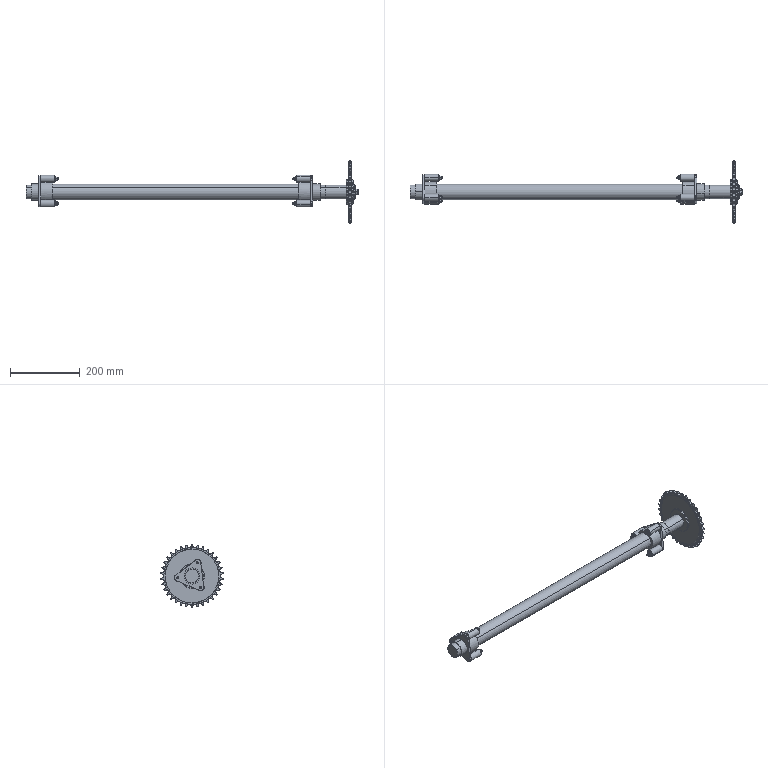Part | SolidWorks | features CompositeCurve 6, AEMSimFeature 1 | 30 solids | 1403 faces | box 950.4 x 178.405 x 179 mm | volume 1880780 mm3 | cone 556 | cylinder 465 | plane 236 | torus 110 | spline 36 | commonest cylinder face diameters 6 x84 14.533 x72 26.567 x72 10.311 x44 10 x37 179 x35